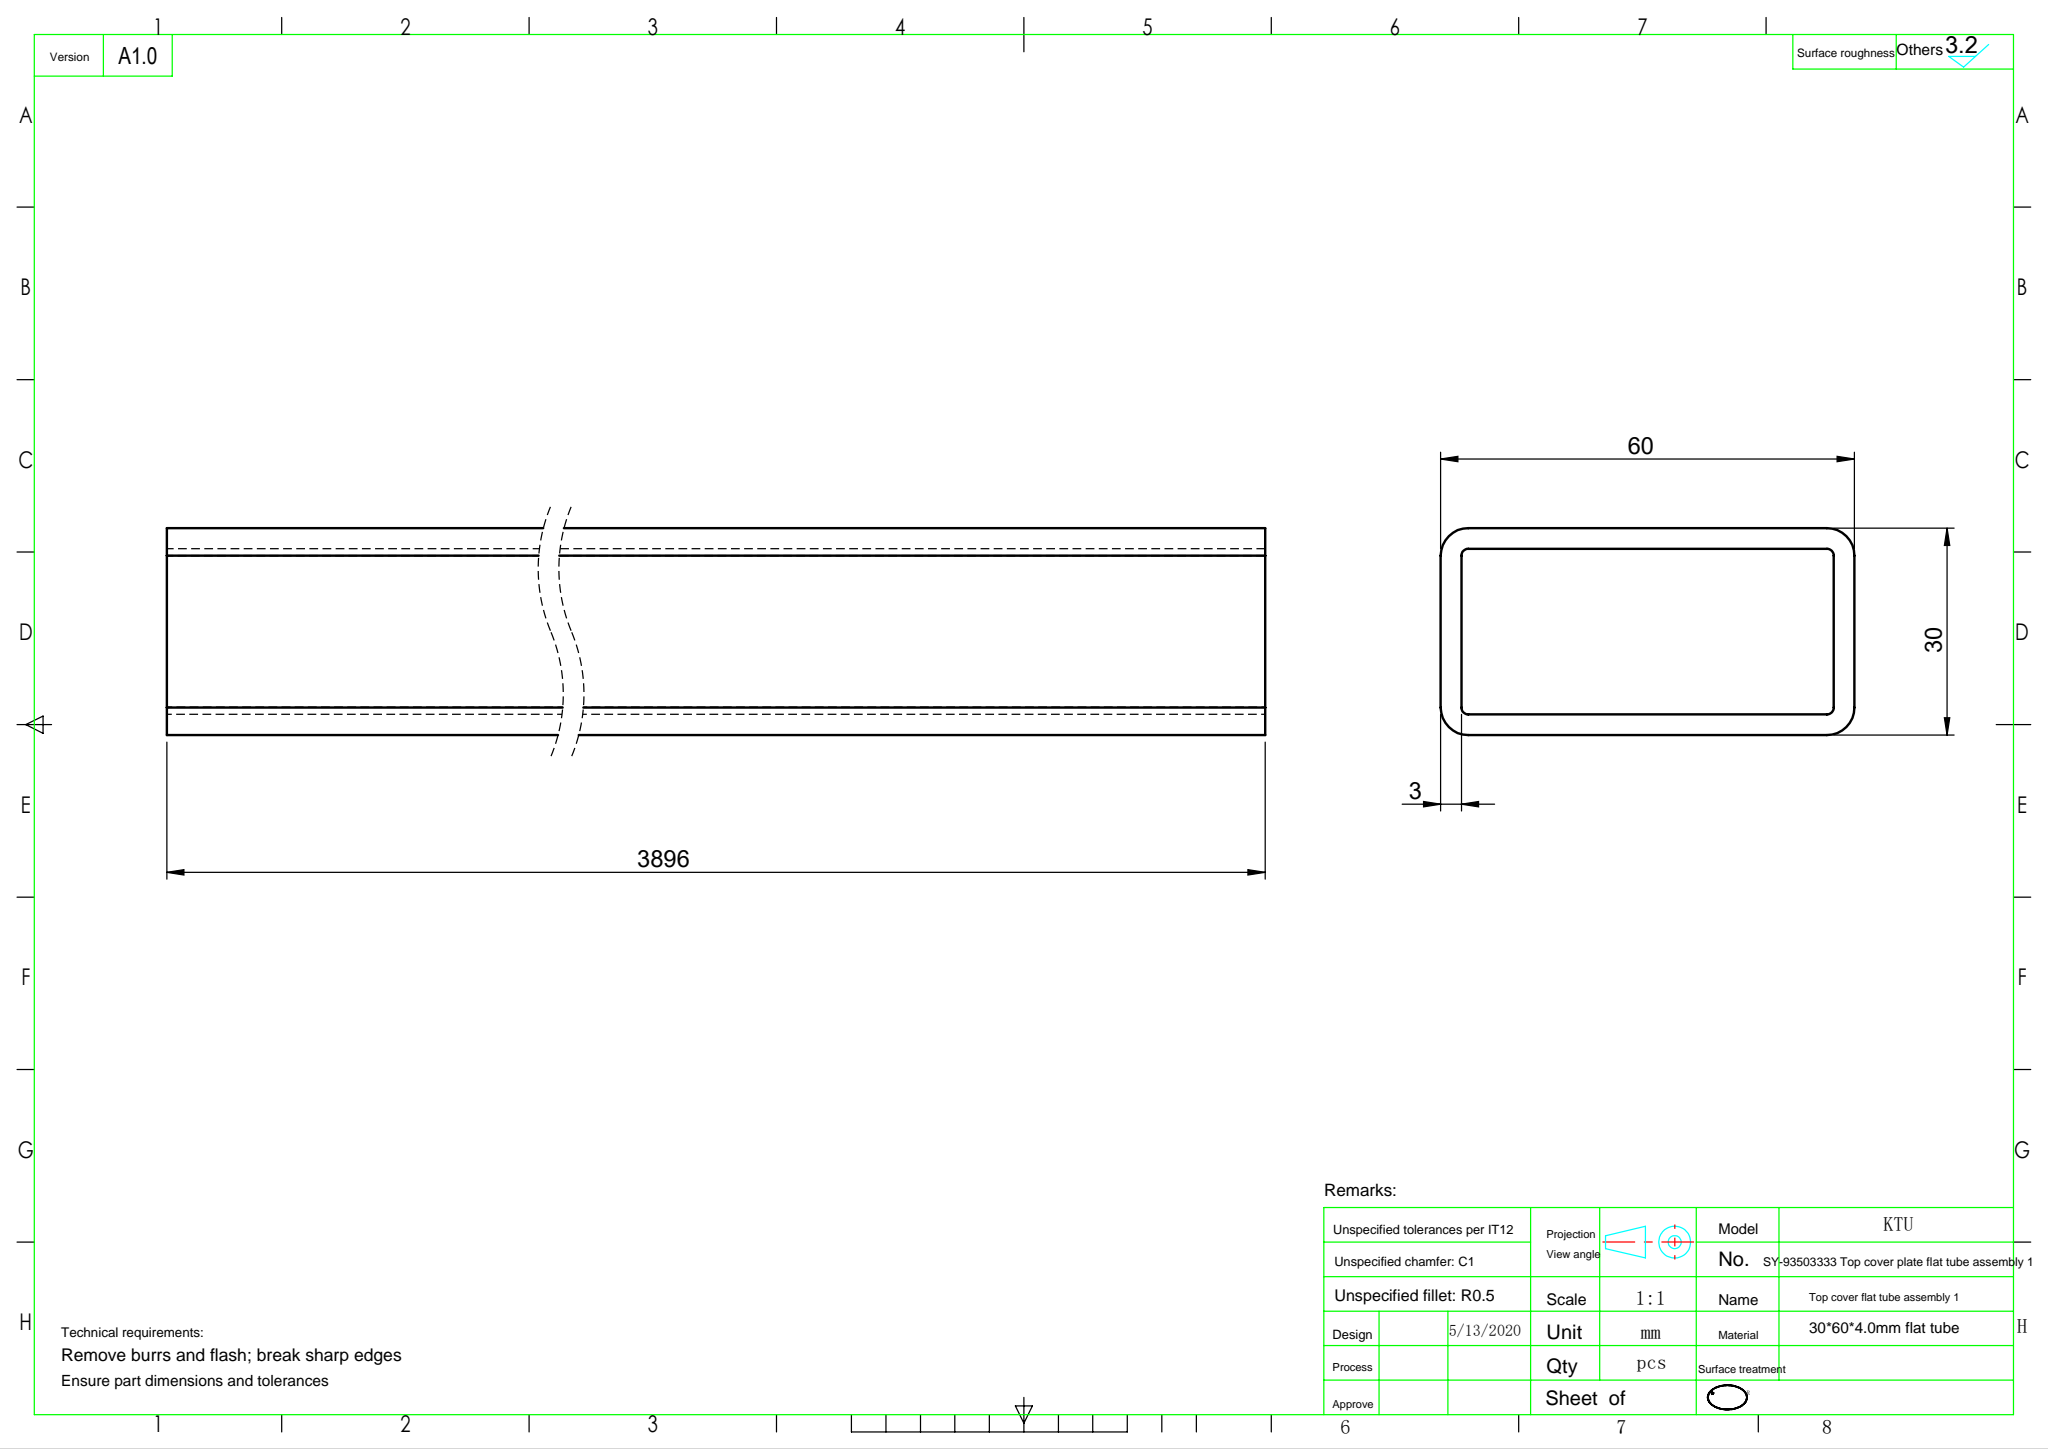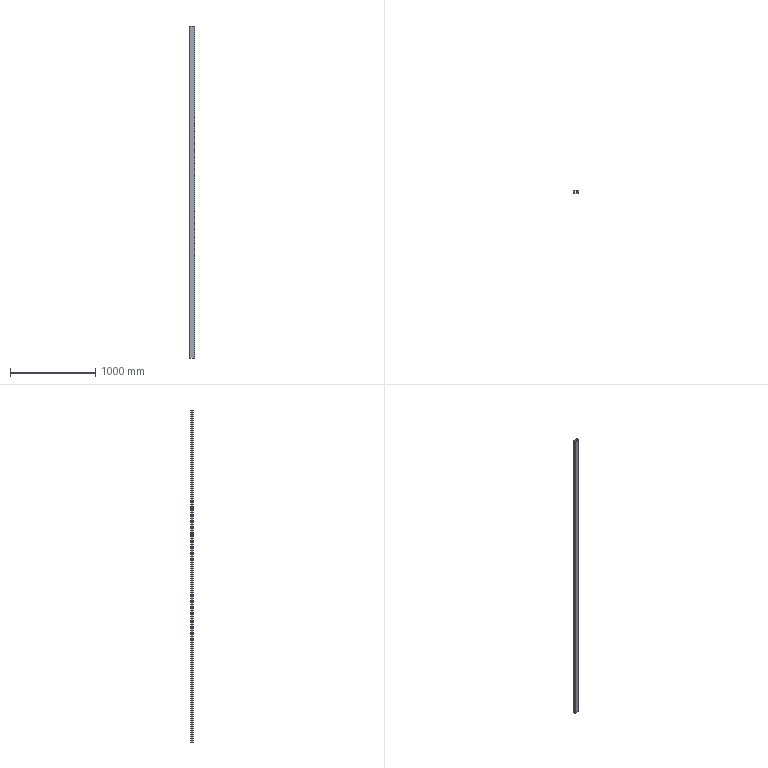Part | SolidWorks | features ExtruThin 1 | 1 solid | 18 faces | box 60 x 30 x 3896 mm | volume 1913419 mm3 | plane 10 | cylinder 8 | commonest cylinder face diameters 2 x4 8 x4
STEP:
#1=CARTESIAN_POINT('',(30.,11.,1948.));
#2=VERTEX_POINT('',#1);
#3=CARTESIAN_POINT('',(26.,15.,1948.));
#4=VERTEX_POINT('',#3);
#5=CARTESIAN_POINT('',(26.,11.,1948.));
#6=DIRECTION('',(0.,0.,1.));
#7=DIRECTION('',(-1.,0.,0.));
#8=AXIS2_PLACEMENT_3D('',#5,#6,#7);
#9=CIRCLE('',#8,4.);
#10=EDGE_CURVE('',#2,#4,#9,.T.);
#11=ORIENTED_EDGE('',*,*,#10,.T.);
#12=CARTESIAN_POINT('',(-26.,15.,1948.));
#13=VERTEX_POINT('',#12);
#14=CARTESIAN_POINT('',(-26.,15.,1948.));
#15=DIRECTION('',(-1.,0.,0.));
#16=VECTOR('',#15,1000.);
#17=LINE('',#14,#16);
#18=EDGE_CURVE('',#4,#13,#17,.T.);
#19=ORIENTED_EDGE('',*,*,#18,.T.);
#20=CARTESIAN_POINT('',(-30.,11.,1948.));
#21=VERTEX_POINT('',#20);
#22=CARTESIAN_POINT('',(-26.,11.,1948.));
#23=DIRECTION('',(0.,0.,1.));
#24=DIRECTION('',(1.,0.,0.));
#25=AXIS2_PLACEMENT_3D('',#22,#23,#24);
#26=CIRCLE('',#25,4.);
#27=EDGE_CURVE('',#13,#21,#26,.T.);
#28=ORIENTED_EDGE('',*,*,#27,.T.);
#29=CARTESIAN_POINT('',(-30.,-11.,1948.));
#30=VERTEX_POINT('',#29);
#31=CARTESIAN_POINT('',(-30.,11.,1948.));
#32=DIRECTION('',(0.,-1.,0.));
#33=VECTOR('',#32,1000.);
#34=LINE('',#31,#33);
#35=EDGE_CURVE('',#21,#30,#34,.T.);
#36=ORIENTED_EDGE('',*,*,#35,.T.);
#37=CARTESIAN_POINT('',(-26.,-15.,1948.));
#38=VERTEX_POINT('',#37);
#39=CARTESIAN_POINT('',(-26.,-11.,1948.));
#40=DIRECTION('',(0.,0.,1.));
#41=DIRECTION('',(1.,0.,0.));
#42=AXIS2_PLACEMENT_3D('',#39,#40,#41);
#43=CIRCLE('',#42,4.);
#44=EDGE_CURVE('',#30,#38,#43,.T.);
#45=ORIENTED_EDGE('',*,*,#44,.T.);
#46=CARTESIAN_POINT('',(26.,-15.,1948.));
#47=VERTEX_POINT('',#46);
#48=CARTESIAN_POINT('',(-26.,-15.,1948.));
#49=DIRECTION('',(1.,0.,0.));
#50=VECTOR('',#49,1000.);
#51=LINE('',#48,#50);
#52=EDGE_CURVE('',#38,#47,#51,.T.);
#53=ORIENTED_EDGE('',*,*,#52,.T.);
#54=CARTESIAN_POINT('',(30.,-11.,1948.));
#55=VERTEX_POINT('',#54);
#56=CARTESIAN_POINT('',(26.,-11.,1948.));
#57=DIRECTION('',(0.,0.,1.));
#58=DIRECTION('',(1.,0.,0.));
#59=AXIS2_PLACEMENT_3D('',#56,#57,#58);
#60=CIRCLE('',#59,4.);
#61=EDGE_CURVE('',#47,#55,#60,.T.);
#62=ORIENTED_EDGE('',*,*,#61,.T.);
#63=CARTESIAN_POINT('',(30.,11.,1948.));
#64=DIRECTION('',(0.,1.,0.));
#65=VECTOR('',#64,1000.);
#66=LINE('',#63,#65);
#67=EDGE_CURVE('',#55,#2,#66,.T.);
#68=ORIENTED_EDGE('',*,*,#67,.T.);
#69=EDGE_LOOP('',(#11,#19,#28,#36,#45,#53,#62,#68));
#70=FACE_OUTER_BOUND('',#69,.T.);
#71=CARTESIAN_POINT('',(26.,12.,1948.));
#72=VERTEX_POINT('',#71);
#73=CARTESIAN_POINT('',(-26.,12.,1948.));
#74=VERTEX_POINT('',#73);
#75=CARTESIAN_POINT('',(26.,12.,1948.));
#76=DIRECTION('',(-1.,0.,0.));
#77=VECTOR('',#76,1000.);
#78=LINE('',#75,#77);
#79=EDGE_CURVE('',#72,#74,#78,.T.);
#80=ORIENTED_EDGE('',*,*,#79,.F.);
#81=CARTESIAN_POINT('',(27.,11.,1948.));
#82=VERTEX_POINT('',#81);
#83=CARTESIAN_POINT('',(26.,11.,1948.));
#84=DIRECTION('',(0.,0.,1.));
#85=DIRECTION('',(-1.,0.,0.));
#86=AXIS2_PLACEMENT_3D('',#83,#84,#85);
#87=CIRCLE('',#86,1.);
#88=EDGE_CURVE('',#82,#72,#87,.T.);
#89=ORIENTED_EDGE('',*,*,#88,.F.);
#90=CARTESIAN_POINT('',(27.,-11.,1948.));
#91=VERTEX_POINT('',#90);
#92=CARTESIAN_POINT('',(27.,11.,1948.));
#93=DIRECTION('',(0.,1.,0.));
#94=VECTOR('',#93,1000.);
#95=LINE('',#92,#94);
#96=EDGE_CURVE('',#91,#82,#95,.T.);
#97=ORIENTED_EDGE('',*,*,#96,.F.);
#98=CARTESIAN_POINT('',(26.,-12.,1948.));
#99=VERTEX_POINT('',#98);
#100=CARTESIAN_POINT('',(26.,-11.,1948.));
#101=DIRECTION('',(0.,0.,1.));
#102=DIRECTION('',(-1.,0.,0.));
#103=AXIS2_PLACEMENT_3D('',#100,#101,#102);
#104=CIRCLE('',#103,1.);
#105=EDGE_CURVE('',#99,#91,#104,.T.);
#106=ORIENTED_EDGE('',*,*,#105,.F.);
#107=CARTESIAN_POINT('',(-26.,-12.,1948.));
#108=VERTEX_POINT('',#107);
#109=CARTESIAN_POINT('',(26.,-12.,1948.));
#110=DIRECTION('',(1.,0.,0.));
#111=VECTOR('',#110,1000.);
#112=LINE('',#109,#111);
#113=EDGE_CURVE('',#108,#99,#112,.T.);
#114=ORIENTED_EDGE('',*,*,#113,.F.);
#115=CARTESIAN_POINT('',(-27.,-11.,1948.));
#116=VERTEX_POINT('',#115);
#117=CARTESIAN_POINT('',(-26.,-11.,1948.));
#118=DIRECTION('',(0.,0.,1.));
#119=DIRECTION('',(-1.,0.,0.));
#120=AXIS2_PLACEMENT_3D('',#117,#118,#119);
#121=CIRCLE('',#120,1.);
#122=EDGE_CURVE('',#116,#108,#121,.T.);
#123=ORIENTED_EDGE('',*,*,#122,.F.);
#124=CARTESIAN_POINT('',(-27.,11.,1948.));
#125=VERTEX_POINT('',#124);
#126=CARTESIAN_POINT('',(-27.,11.,1948.));
#127=DIRECTION('',(0.,-1.,0.));
#128=VECTOR('',#127,1000.);
#129=LINE('',#126,#128);
#130=EDGE_CURVE('',#125,#116,#129,.T.);
#131=ORIENTED_EDGE('',*,*,#130,.F.);
#132=CARTESIAN_POINT('',(-26.,11.,1948.));
#133=DIRECTION('',(0.,0.,1.));
#134=DIRECTION('',(-1.,0.,0.));
#135=AXIS2_PLACEMENT_3D('',#132,#133,#134);
#136=CIRCLE('',#135,1.);
#137=EDGE_CURVE('',#74,#125,#136,.T.);
#138=ORIENTED_EDGE('',*,*,#137,.F.);
#139=EDGE_LOOP('',(#80,#89,#97,#106,#114,#123,#131,#138));
#140=FACE_BOUND('',#139,.T.);
#141=CARTESIAN_POINT('',(26.,11.,1948.));
#142=DIRECTION('',(0.,0.,1.));
#143=DIRECTION('',(1.,0.,0.));
#144=AXIS2_PLACEMENT_3D('',#141,#142,#143);
#145=PLANE('',#144);
#146=ADVANCED_FACE('',(#70,#140),#145,.T.);
#147=CARTESIAN_POINT('',(30.,11.,-1948.));
#148=VERTEX_POINT('',#147);
#149=CARTESIAN_POINT('',(26.,15.,-1948.));
#150=VERTEX_POINT('',#149);
#151=CARTESIAN_POINT('',(26.,11.,-1948.));
#152=DIRECTION('',(0.,0.,1.));
#153=DIRECTION('',(-1.,0.,0.));
#154=AXIS2_PLACEMENT_3D('',#151,#152,#153);
#155=CIRCLE('',#154,4.);
#156=EDGE_CURVE('',#148,#150,#155,.T.);
#157=ORIENTED_EDGE('',*,*,#156,.F.);
#158=CARTESIAN_POINT('',(30.,-11.,-1948.));
#159=VERTEX_POINT('',#158);
#160=CARTESIAN_POINT('',(30.,11.,-1948.));
#161=DIRECTION('',(0.,1.,0.));
#162=VECTOR('',#161,1000.);
#163=LINE('',#160,#162);
#164=EDGE_CURVE('',#159,#148,#163,.T.);
#165=ORIENTED_EDGE('',*,*,#164,.F.);
#166=CARTESIAN_POINT('',(26.,-15.,-1948.));
#167=VERTEX_POINT('',#166);
#168=CARTESIAN_POINT('',(26.,-11.,-1948.));
#169=DIRECTION('',(0.,0.,1.));
#170=DIRECTION('',(1.,0.,0.));
#171=AXIS2_PLACEMENT_3D('',#168,#169,#170);
#172=CIRCLE('',#171,4.);
#173=EDGE_CURVE('',#167,#159,#172,.T.);
#174=ORIENTED_EDGE('',*,*,#173,.F.);
#175=CARTESIAN_POINT('',(-26.,-15.,-1948.));
#176=VERTEX_POINT('',#175);
#177=CARTESIAN_POINT('',(-26.,-15.,-1948.));
#178=DIRECTION('',(1.,0.,0.));
#179=VECTOR('',#178,1000.);
#180=LINE('',#177,#179);
#181=EDGE_CURVE('',#176,#167,#180,.T.);
#182=ORIENTED_EDGE('',*,*,#181,.F.);
#183=CARTESIAN_POINT('',(-30.,-11.,-1948.));
#184=VERTEX_POINT('',#183);
#185=CARTESIAN_POINT('',(-26.,-11.,-1948.));
#186=DIRECTION('',(0.,0.,1.));
#187=DIRECTION('',(1.,0.,0.));
#188=AXIS2_PLACEMENT_3D('',#185,#186,#187);
#189=CIRCLE('',#188,4.);
#190=EDGE_CURVE('',#184,#176,#189,.T.);
#191=ORIENTED_EDGE('',*,*,#190,.F.);
#192=CARTESIAN_POINT('',(-30.,11.,-1948.));
#193=VERTEX_POINT('',#192);
#194=CARTESIAN_POINT('',(-30.,11.,-1948.));
#195=DIRECTION('',(0.,-1.,0.));
#196=VECTOR('',#195,1000.);
#197=LINE('',#194,#196);
#198=EDGE_CURVE('',#193,#184,#197,.T.);
#199=ORIENTED_EDGE('',*,*,#198,.F.);
#200=CARTESIAN_POINT('',(-26.,15.,-1948.));
#201=VERTEX_POINT('',#200);
#202=CARTESIAN_POINT('',(-26.,11.,-1948.));
#203=DIRECTION('',(0.,0.,1.));
#204=DIRECTION('',(1.,0.,0.));
#205=AXIS2_PLACEMENT_3D('',#202,#203,#204);
#206=CIRCLE('',#205,4.);
#207=EDGE_CURVE('',#201,#193,#206,.T.);
#208=ORIENTED_EDGE('',*,*,#207,.F.);
#209=CARTESIAN_POINT('',(-26.,15.,-1948.));
#210=DIRECTION('',(-1.,0.,0.));
#211=VECTOR('',#210,1000.);
#212=LINE('',#209,#211);
#213=EDGE_CURVE('',#150,#201,#212,.T.);
#214=ORIENTED_EDGE('',*,*,#213,.F.);
#215=EDGE_LOOP('',(#157,#165,#174,#182,#191,#199,#208,#214));
#216=FACE_OUTER_BOUND('',#215,.T.);
#217=CARTESIAN_POINT('',(27.,11.,-1948.));
#218=VERTEX_POINT('',#217);
#219=CARTESIAN_POINT('',(26.,12.,-1948.));
#220=VERTEX_POINT('',#219);
#221=CARTESIAN_POINT('',(26.,11.,-1948.));
#222=DIRECTION('',(0.,0.,1.));
#223=DIRECTION('',(-1.,0.,0.));
#224=AXIS2_PLACEMENT_3D('',#221,#222,#223);
#225=CIRCLE('',#224,1.);
#226=EDGE_CURVE('',#218,#220,#225,.T.);
#227=ORIENTED_EDGE('',*,*,#226,.T.);
#228=CARTESIAN_POINT('',(-26.,12.,-1948.));
#229=VERTEX_POINT('',#228);
#230=CARTESIAN_POINT('',(26.,12.,-1948.));
#231=DIRECTION('',(-1.,0.,0.));
#232=VECTOR('',#231,1000.);
#233=LINE('',#230,#232);
#234=EDGE_CURVE('',#220,#229,#233,.T.);
#235=ORIENTED_EDGE('',*,*,#234,.T.);
#236=CARTESIAN_POINT('',(-27.,11.,-1948.));
#237=VERTEX_POINT('',#236);
#238=CARTESIAN_POINT('',(-26.,11.,-1948.));
#239=DIRECTION('',(0.,0.,1.));
#240=DIRECTION('',(-1.,0.,0.));
#241=AXIS2_PLACEMENT_3D('',#238,#239,#240);
#242=CIRCLE('',#241,1.);
#243=EDGE_CURVE('',#229,#237,#242,.T.);
#244=ORIENTED_EDGE('',*,*,#243,.T.);
#245=CARTESIAN_POINT('',(-27.,-11.,-1948.));
#246=VERTEX_POINT('',#245);
#247=CARTESIAN_POINT('',(-27.,11.,-1948.));
#248=DIRECTION('',(0.,-1.,0.));
#249=VECTOR('',#248,1000.);
#250=LINE('',#247,#249);
#251=EDGE_CURVE('',#237,#246,#250,.T.);
#252=ORIENTED_EDGE('',*,*,#251,.T.);
#253=CARTESIAN_POINT('',(-26.,-12.,-1948.));
#254=VERTEX_POINT('',#253);
#255=CARTESIAN_POINT('',(-26.,-11.,-1948.));
#256=DIRECTION('',(0.,0.,1.));
#257=DIRECTION('',(-1.,0.,0.));
#258=AXIS2_PLACEMENT_3D('',#255,#256,#257);
#259=CIRCLE('',#258,1.);
#260=EDGE_CURVE('',#246,#254,#259,.T.);
#261=ORIENTED_EDGE('',*,*,#260,.T.);
#262=CARTESIAN_POINT('',(26.,-12.,-1948.));
#263=VERTEX_POINT('',#262);
#264=CARTESIAN_POINT('',(26.,-12.,-1948.));
#265=DIRECTION('',(1.,0.,0.));
#266=VECTOR('',#265,1000.);
#267=LINE('',#264,#266);
#268=EDGE_CURVE('',#254,#263,#267,.T.);
#269=ORIENTED_EDGE('',*,*,#268,.T.);
#270=CARTESIAN_POINT('',(27.,-11.,-1948.));
#271=VERTEX_POINT('',#270);
#272=CARTESIAN_POINT('',(26.,-11.,-1948.));
#273=DIRECTION('',(0.,0.,1.));
#274=DIRECTION('',(-1.,0.,0.));
#275=AXIS2_PLACEMENT_3D('',#272,#273,#274);
#276=CIRCLE('',#275,1.);
#277=EDGE_CURVE('',#263,#271,#276,.T.);
#278=ORIENTED_EDGE('',*,*,#277,.T.);
#279=CARTESIAN_POINT('',(27.,11.,-1948.));
#280=DIRECTION('',(0.,1.,0.));
#281=VECTOR('',#280,1000.);
#282=LINE('',#279,#281);
#283=EDGE_CURVE('',#271,#218,#282,.T.);
#284=ORIENTED_EDGE('',*,*,#283,.T.);
#285=EDGE_LOOP('',(#227,#235,#244,#252,#261,#269,#278,#284));
#286=FACE_BOUND('',#285,.T.);
#287=CARTESIAN_POINT('',(26.,11.,-1948.));
#288=DIRECTION('',(0.,0.,1.));
#289=DIRECTION('',(1.,0.,0.));
#290=AXIS2_PLACEMENT_3D('',#287,#288,#289);
#291=PLANE('',#290);
#292=ADVANCED_FACE('',(#216,#286),#291,.F.);
#293=ORIENTED_EDGE('',*,*,#156,.T.);
#294=CARTESIAN_POINT('',(26.,15.,1948.));
#295=DIRECTION('',(0.,0.,-1.));
#296=VECTOR('',#295,1000.);
#297=LINE('',#294,#296);
#298=EDGE_CURVE('',#4,#150,#297,.T.);
#299=ORIENTED_EDGE('',*,*,#298,.F.);
#300=ORIENTED_EDGE('',*,*,#10,.F.);
#301=CARTESIAN_POINT('',(30.,11.,1948.));
#302=DIRECTION('',(0.,0.,-1.));
#303=VECTOR('',#302,1000.);
#304=LINE('',#301,#303);
#305=EDGE_CURVE('',#2,#148,#304,.T.);
#306=ORIENTED_EDGE('',*,*,#305,.T.);
#307=EDGE_LOOP('',(#293,#299,#300,#306));
#308=FACE_OUTER_BOUND('',#307,.T.);
#309=CARTESIAN_POINT('',(26.,11.,1948.));
#310=DIRECTION('',(0.,0.,-1.));
#311=DIRECTION('',(-1.,0.,0.));
#312=AXIS2_PLACEMENT_3D('',#309,#310,#311);
#313=CYLINDRICAL_SURFACE('',#312,4.);
#314=ADVANCED_FACE('',(#308),#313,.T.);
#315=ORIENTED_EDGE('',*,*,#213,.T.);
#316=CARTESIAN_POINT('',(-26.,15.,1948.));
#317=DIRECTION('',(0.,0.,-1.));
#318=VECTOR('',#317,1000.);
#319=LINE('',#316,#318);
#320=EDGE_CURVE('',#13,#201,#319,.T.);
#321=ORIENTED_EDGE('',*,*,#320,.F.);
#322=ORIENTED_EDGE('',*,*,#18,.F.);
#323=ORIENTED_EDGE('',*,*,#298,.T.);
#324=EDGE_LOOP('',(#315,#321,#322,#323));
#325=FACE_OUTER_BOUND('',#324,.T.);
#326=CARTESIAN_POINT('',(-26.,15.,1948.));
#327=DIRECTION('',(0.,-1.,0.));
#328=DIRECTION('',(0.,0.,-1.));
#329=AXIS2_PLACEMENT_3D('',#326,#327,#328);
#330=PLANE('',#329);
#331=ADVANCED_FACE('',(#325),#330,.F.);
#332=ORIENTED_EDGE('',*,*,#207,.T.);
#333=CARTESIAN_POINT('',(-30.,11.,1948.));
#334=DIRECTION('',(0.,0.,-1.));
#335=VECTOR('',#334,1000.);
#336=LINE('',#333,#335);
#337=EDGE_CURVE('',#21,#193,#336,.T.);
#338=ORIENTED_EDGE('',*,*,#337,.F.);
#339=ORIENTED_EDGE('',*,*,#27,.F.);
#340=ORIENTED_EDGE('',*,*,#320,.T.);
#341=EDGE_LOOP('',(#332,#338,#339,#340));
#342=FACE_OUTER_BOUND('',#341,.T.);
#343=CARTESIAN_POINT('',(-26.,11.,1948.));
#344=DIRECTION('',(0.,0.,-1.));
#345=DIRECTION('',(-1.,0.,0.));
#346=AXIS2_PLACEMENT_3D('',#343,#344,#345);
#347=CYLINDRICAL_SURFACE('',#346,4.);
#348=ADVANCED_FACE('',(#342),#347,.T.);
#349=ORIENTED_EDGE('',*,*,#198,.T.);
#350=CARTESIAN_POINT('',(-30.,-11.,1948.));
#351=DIRECTION('',(0.,0.,-1.));
#352=VECTOR('',#351,1000.);
#353=LINE('',#350,#352);
#354=EDGE_CURVE('',#30,#184,#353,.T.);
#355=ORIENTED_EDGE('',*,*,#354,.F.);
#356=ORIENTED_EDGE('',*,*,#35,.F.);
#357=ORIENTED_EDGE('',*,*,#337,.T.);
#358=EDGE_LOOP('',(#349,#355,#356,#357));
#359=FACE_OUTER_BOUND('',#358,.T.);
#360=CARTESIAN_POINT('',(-30.,11.,1948.));
#361=DIRECTION('',(1.,0.,0.));
#362=DIRECTION('',(0.,1.,0.));
#363=AXIS2_PLACEMENT_3D('',#360,#361,#362);
#364=PLANE('',#363);
#365=ADVANCED_FACE('',(#359),#364,.F.);
#366=ORIENTED_EDGE('',*,*,#190,.T.);
#367=CARTESIAN_POINT('',(-26.,-15.,1948.));
#368=DIRECTION('',(0.,0.,-1.));
#369=VECTOR('',#368,1000.);
#370=LINE('',#367,#369);
#371=EDGE_CURVE('',#38,#176,#370,.T.);
#372=ORIENTED_EDGE('',*,*,#371,.F.);
#373=ORIENTED_EDGE('',*,*,#44,.F.);
#374=ORIENTED_EDGE('',*,*,#354,.T.);
#375=EDGE_LOOP('',(#366,#372,#373,#374));
#376=FACE_OUTER_BOUND('',#375,.T.);
#377=CARTESIAN_POINT('',(-26.,-11.,1948.));
#378=DIRECTION('',(0.,0.,-1.));
#379=DIRECTION('',(-1.,0.,0.));
#380=AXIS2_PLACEMENT_3D('',#377,#378,#379);
#381=CYLINDRICAL_SURFACE('',#380,4.);
#382=ADVANCED_FACE('',(#376),#381,.T.);
#383=ORIENTED_EDGE('',*,*,#181,.T.);
#384=CARTESIAN_POINT('',(26.,-15.,1948.));
#385=DIRECTION('',(0.,0.,-1.));
#386=VECTOR('',#385,1000.);
#387=LINE('',#384,#386);
#388=EDGE_CURVE('',#47,#167,#387,.T.);
#389=ORIENTED_EDGE('',*,*,#388,.F.);
#390=ORIENTED_EDGE('',*,*,#52,.F.);
#391=ORIENTED_EDGE('',*,*,#371,.T.);
#392=EDGE_LOOP('',(#383,#389,#390,#391));
#393=FACE_OUTER_BOUND('',#392,.T.);
#394=CARTESIAN_POINT('',(-26.,-15.,1948.));
#395=DIRECTION('',(0.,1.,0.));
#396=DIRECTION('',(0.,0.,1.));
#397=AXIS2_PLACEMENT_3D('',#394,#395,#396);
#398=PLANE('',#397);
#399=ADVANCED_FACE('',(#393),#398,.F.);
#400=ORIENTED_EDGE('',*,*,#173,.T.);
#401=CARTESIAN_POINT('',(30.,-11.,1948.));
#402=DIRECTION('',(0.,0.,-1.));
#403=VECTOR('',#402,1000.);
#404=LINE('',#401,#403);
#405=EDGE_CURVE('',#55,#159,#404,.T.);
#406=ORIENTED_EDGE('',*,*,#405,.F.);
#407=ORIENTED_EDGE('',*,*,#61,.F.);
#408=ORIENTED_EDGE('',*,*,#388,.T.);
#409=EDGE_LOOP('',(#400,#406,#407,#408));
#410=FACE_OUTER_BOUND('',#409,.T.);
#411=CARTESIAN_POINT('',(26.,-11.,1948.));
#412=DIRECTION('',(0.,0.,-1.));
#413=DIRECTION('',(-1.,0.,0.));
#414=AXIS2_PLACEMENT_3D('',#411,#412,#413);
#415=CYLINDRICAL_SURFACE('',#414,4.);
#416=ADVANCED_FACE('',(#410),#415,.T.);
#417=ORIENTED_EDGE('',*,*,#164,.T.);
#418=ORIENTED_EDGE('',*,*,#305,.F.);
#419=ORIENTED_EDGE('',*,*,#67,.F.);
#420=ORIENTED_EDGE('',*,*,#405,.T.);
#421=EDGE_LOOP('',(#417,#418,#419,#420));
#422=FACE_OUTER_BOUND('',#421,.T.);
#423=CARTESIAN_POINT('',(30.,11.,1948.));
#424=DIRECTION('',(-1.,0.,0.));
#425=DIRECTION('',(0.,-1.,0.));
#426=AXIS2_PLACEMENT_3D('',#423,#424,#425);
#427=PLANE('',#426);
#428=ADVANCED_FACE('',(#422),#427,.F.);
#429=ORIENTED_EDGE('',*,*,#226,.F.);
#430=CARTESIAN_POINT('',(27.,11.,1948.));
#431=DIRECTION('',(0.,0.,-1.));
#432=VECTOR('',#431,1000.);
#433=LINE('',#430,#432);
#434=EDGE_CURVE('',#82,#218,#433,.T.);
#435=ORIENTED_EDGE('',*,*,#434,.F.);
#436=ORIENTED_EDGE('',*,*,#88,.T.);
#437=CARTESIAN_POINT('',(26.,12.,1948.));
#438=DIRECTION('',(0.,0.,-1.));
#439=VECTOR('',#438,1000.);
#440=LINE('',#437,#439);
#441=EDGE_CURVE('',#72,#220,#440,.T.);
#442=ORIENTED_EDGE('',*,*,#441,.T.);
#443=EDGE_LOOP('',(#429,#435,#436,#442));
#444=FACE_OUTER_BOUND('',#443,.T.);
#445=CARTESIAN_POINT('',(26.,11.,1948.));
#446=DIRECTION('',(0.,0.,-1.));
#447=DIRECTION('',(-1.,0.,0.));
#448=AXIS2_PLACEMENT_3D('',#445,#446,#447);
#449=CYLINDRICAL_SURFACE('',#448,1.);
#450=ADVANCED_FACE('',(#444),#449,.F.);
#451=ORIENTED_EDGE('',*,*,#234,.F.);
#452=ORIENTED_EDGE('',*,*,#441,.F.);
#453=ORIENTED_EDGE('',*,*,#79,.T.);
#454=CARTESIAN_POINT('',(-26.,12.,1948.));
#455=DIRECTION('',(0.,0.,-1.));
#456=VECTOR('',#455,1000.);
#457=LINE('',#454,#456);
#458=EDGE_CURVE('',#74,#229,#457,.T.);
#459=ORIENTED_EDGE('',*,*,#458,.T.);
#460=EDGE_LOOP('',(#451,#452,#453,#459));
#461=FACE_OUTER_BOUND('',#460,.T.);
#462=CARTESIAN_POINT('',(26.,12.,1948.));
#463=DIRECTION('',(0.,-1.,0.));
#464=DIRECTION('',(0.,0.,-1.));
#465=AXIS2_PLACEMENT_3D('',#462,#463,#464);
#466=PLANE('',#465);
#467=ADVANCED_FACE('',(#461),#466,.T.);
#468=ORIENTED_EDGE('',*,*,#243,.F.);
#469=ORIENTED_EDGE('',*,*,#458,.F.);
#470=ORIENTED_EDGE('',*,*,#137,.T.);
#471=CARTESIAN_POINT('',(-27.,11.,1948.));
#472=DIRECTION('',(0.,0.,-1.));
#473=VECTOR('',#472,1000.);
#474=LINE('',#471,#473);
#475=EDGE_CURVE('',#125,#237,#474,.T.);
#476=ORIENTED_EDGE('',*,*,#475,.T.);
#477=EDGE_LOOP('',(#468,#469,#470,#476));
#478=FACE_OUTER_BOUND('',#477,.T.);
#479=CARTESIAN_POINT('',(-26.,11.,1948.));
#480=DIRECTION('',(0.,0.,-1.));
#481=DIRECTION('',(-1.,0.,0.));
#482=AXIS2_PLACEMENT_3D('',#479,#480,#481);
#483=CYLINDRICAL_SURFACE('',#482,1.);
#484=ADVANCED_FACE('',(#478),#483,.F.);
#485=ORIENTED_EDGE('',*,*,#251,.F.);
#486=ORIENTED_EDGE('',*,*,#475,.F.);
#487=ORIENTED_EDGE('',*,*,#130,.T.);
#488=CARTESIAN_POINT('',(-27.,-11.,1948.));
#489=DIRECTION('',(0.,0.,-1.));
#490=VECTOR('',#489,1000.);
#491=LINE('',#488,#490);
#492=EDGE_CURVE('',#116,#246,#491,.T.);
#493=ORIENTED_EDGE('',*,*,#492,.T.);
#494=EDGE_LOOP('',(#485,#486,#487,#493));
#495=FACE_OUTER_BOUND('',#494,.T.);
#496=CARTESIAN_POINT('',(-27.,11.,1948.));
#497=DIRECTION('',(1.,0.,0.));
#498=DIRECTION('',(0.,1.,0.));
#499=AXIS2_PLACEMENT_3D('',#496,#497,#498);
#500=PLANE('',#499);
#501=ADVANCED_FACE('',(#495),#500,.T.);
#502=ORIENTED_EDGE('',*,*,#260,.F.);
#503=ORIENTED_EDGE('',*,*,#492,.F.);
#504=ORIENTED_EDGE('',*,*,#122,.T.);
#505=CARTESIAN_POINT('',(-26.,-12.,1948.));
#506=DIRECTION('',(0.,0.,-1.));
#507=VECTOR('',#506,1000.);
#508=LINE('',#505,#507);
#509=EDGE_CURVE('',#108,#254,#508,.T.);
#510=ORIENTED_EDGE('',*,*,#509,.T.);
#511=EDGE_LOOP('',(#502,#503,#504,#510));
#512=FACE_OUTER_BOUND('',#511,.T.);
#513=CARTESIAN_POINT('',(-26.,-11.,1948.));
#514=DIRECTION('',(0.,0.,-1.));
#515=DIRECTION('',(-1.,0.,0.));
#516=AXIS2_PLACEMENT_3D('',#513,#514,#515);
#517=CYLINDRICAL_SURFACE('',#516,1.);
#518=ADVANCED_FACE('',(#512),#517,.F.);
#519=ORIENTED_EDGE('',*,*,#268,.F.);
#520=ORIENTED_EDGE('',*,*,#509,.F.);
#521=ORIENTED_EDGE('',*,*,#113,.T.);
#522=CARTESIAN_POINT('',(26.,-12.,1948.));
#523=DIRECTION('',(0.,0.,-1.));
#524=VECTOR('',#523,1000.);
#525=LINE('',#522,#524);
#526=EDGE_CURVE('',#99,#263,#525,.T.);
#527=ORIENTED_EDGE('',*,*,#526,.T.);
#528=EDGE_LOOP('',(#519,#520,#521,#527));
#529=FACE_OUTER_BOUND('',#528,.T.);
#530=CARTESIAN_POINT('',(26.,-12.,1948.));
#531=DIRECTION('',(0.,1.,0.));
#532=DIRECTION('',(0.,0.,1.));
#533=AXIS2_PLACEMENT_3D('',#530,#531,#532);
#534=PLANE('',#533);
#535=ADVANCED_FACE('',(#529),#534,.T.);
#536=ORIENTED_EDGE('',*,*,#277,.F.);
#537=ORIENTED_EDGE('',*,*,#526,.F.);
#538=ORIENTED_EDGE('',*,*,#105,.T.);
#539=CARTESIAN_POINT('',(27.,-11.,1948.));
#540=DIRECTION('',(0.,0.,-1.));
#541=VECTOR('',#540,1000.);
#542=LINE('',#539,#541);
#543=EDGE_CURVE('',#91,#271,#542,.T.);
#544=ORIENTED_EDGE('',*,*,#543,.T.);
#545=EDGE_LOOP('',(#536,#537,#538,#544));
#546=FACE_OUTER_BOUND('',#545,.T.);
#547=CARTESIAN_POINT('',(26.,-11.,1948.));
#548=DIRECTION('',(0.,0.,-1.));
#549=DIRECTION('',(-1.,0.,0.));
#550=AXIS2_PLACEMENT_3D('',#547,#548,#549);
#551=CYLINDRICAL_SURFACE('',#550,1.);
#552=ADVANCED_FACE('',(#546),#551,.F.);
#553=ORIENTED_EDGE('',*,*,#283,.F.);
#554=ORIENTED_EDGE('',*,*,#543,.F.);
#555=ORIENTED_EDGE('',*,*,#96,.T.);
#556=ORIENTED_EDGE('',*,*,#434,.T.);
#557=EDGE_LOOP('',(#553,#554,#555,#556));
#558=FACE_OUTER_BOUND('',#557,.T.);
#559=CARTESIAN_POINT('',(27.,11.,1948.));
#560=DIRECTION('',(-1.,0.,0.));
#561=DIRECTION('',(0.,-1.,0.));
#562=AXIS2_PLACEMENT_3D('',#559,#560,#561);
#563=PLANE('',#562);
#564=ADVANCED_FACE('',(#558),#563,.T.);
#565=CLOSED_SHELL('',(#146,#292,#314,#331,#348,#365,#382,#399,#416,#428,#450,#467,#484,#501,#518,#535,#552,#564));
#566=MANIFOLD_SOLID_BREP('',#565);
#567=CARTESIAN_POINT('',(0.,0.,0.));
#568=DIRECTION('',(0.,0.,1.));
#569=DIRECTION('',(1.,0.,0.));
#570=AXIS2_PLACEMENT_3D('',#567,#568,#569);
#571=(LENGTH_UNIT()NAMED_UNIT(*)SI_UNIT(.MILLI.,.METRE.));
#572=UNCERTAINTY_MEASURE_WITH_UNIT(LENGTH_MEASURE(0.00001),#571,'','');
#573=(NAMED_UNIT(*)PLANE_ANGLE_UNIT()SI_UNIT($,.RADIAN.));
#574=(NAMED_UNIT(*)SI_UNIT($,.STERADIAN.)SOLID_ANGLE_UNIT());
#575=(GEOMETRIC_REPRESENTATION_CONTEXT(3)GLOBAL_UNCERTAINTY_ASSIGNED_CONTEXT((#572))GLOBAL_UNIT_ASSIGNED_CONTEXT((#571,#573,#574))REPRESENTATION_CONTEXT('',''));
#576=ADVANCED_BREP_SHAPE_REPRESENTATION('',(#566,#570),#575);